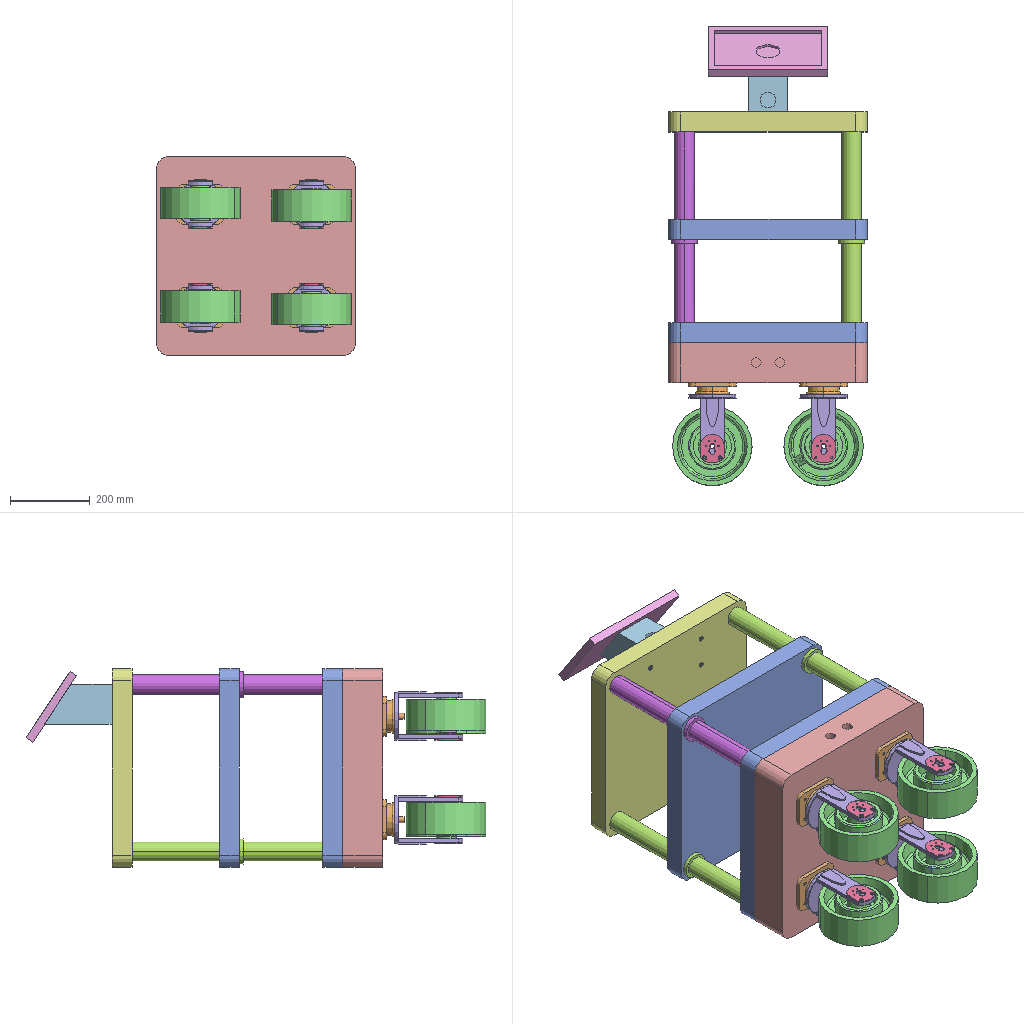Assembly | SolidWorks | 13 different items | 35 placed | box 500 x 1156 x 500 mm
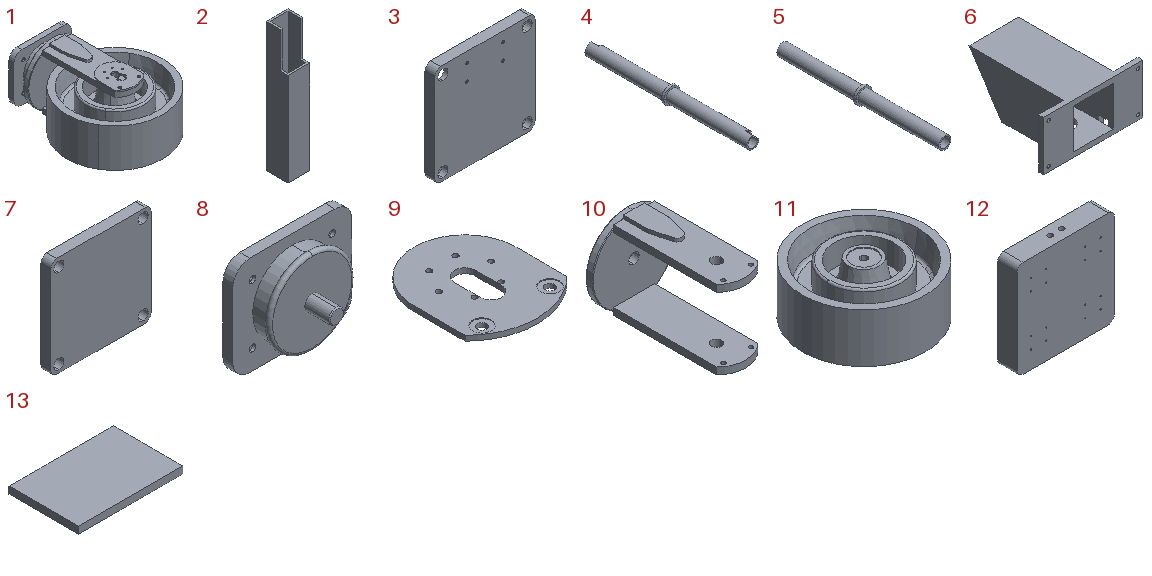Parts list (item | name | quantity | parent item | size | volume | features):
1 | (subassembly) | x4 | - | 200 x 260 x 124 mm | 1930087 mm3 | features CompositeCurve 10, AEMSimFeature 1, MirrorCompFeat 1, ReferencePattern 1
2 | - | x1 | - | 30 x 30 x 180 mm | 43875 mm3 | features ICE 2, Extrusion 1
3 | - | x1 | - | 500 x 50 x 500 mm | 7022317 mm3 | features ICE 3, Extrusion 1, HoleWzd 1
4 | - | x1 | - | 66 x 660 x 66 mm | 470501 mm3 | features ICE 3, Revolution 1
5 | - | x3 | - | 66 x 660 x 66 mm | 481103 mm3 | features ICE 1, Revolution 1
6 | - | x1 | - | 200 x 200 x 100 mm | 682330 mm3 | features ICE 4, Extrusion 1, HoleWzd 1
7 | - | x2 | - | 500 x 50 x 500 mm | 6892126 mm3 | features ICE 2, Extrusion 1
8 | - | x4 | in 1 | 120 x 55 x 100 mm | 210377 mm3 | features ICE 3, Chamfer 1, Extrusion 1, HoleWzd 1, Revolution 1
9 | - | x8 | in 1 | 60 x 72.426 x 3 mm | 9913 mm3 | features Extrusion 1, HoleWzd 1, ICE 1
10 | - | x4 | in 1 | 120 x 172.426 x 124 mm | 314917 mm3 | features ICE 3, MirrorPattern 2, Extrusion 1, Fillet 1, HoleWzd 1
11 | - | x4 | in 1 | 200 x 200 x 87 mm | 1384967 mm3 | features ICE 3, Fillet 2, Extrusion 1, Revolution 1
12 | - | x1 | - | 500 x 100 x 500 mm | 10401596 mm3 | features ICE 4, 3DProfileFeature 1, Extrusion 1, HoleWzd 1, MirrorPattern 1
13 | - | x1 | - | 300 x 200 x 20 mm | 751035 mm3 | features ICE 2, Extrusion 1
Mates (type | each side: item.copy, entity, surface, feature):
In the top assembly
Coincident | 12.1 face plane Cut-Extrude2 | 5.1 face plane Revolve1
Concentric | 12.1 face cylinder Cut-Extrude2 | 5.1 face cylinder Revolve1
Coincident | 12.1 face plane Cut-Extrude1 | assembly face
Concentric | 12.1 face cylinder Cut-Extrude2 | assembly face
Coincident | 12.1 face plane Cut-Extrude2 | 5.2 edge
Concentric | 12.1 face cylinder Cut-Extrude2 | 5.2 face cylinder Revolve1
Coincident | 12.1 face plane Cut-Extrude2 | 5.3 face plane Revolve1
Concentric | 12.1 face cylinder Cut-Extrude2 | 5.3 face cylinder Revolve1
Coincident | 12.1 face plane Boss-Extrude1 | 7.1 face plane Boss-Extrude1
Concentric | 7.1 face cylinder Cut-Extrude2 | assembly face
Concentric | 7.1 face cylinder Cut-Extrude2 | 5.1 face cylinder Revolve1
Concentric | 7.2 face cylinder Cut-Extrude2 | assembly face
Concentric | 7.2 face cylinder Cut-Extrude2 | 5.2 face cylinder Revolve1
Coincident | 5.1 face plane Revolve1 | 7.2 face plane Boss-Extrude1
Coincident | 12.1 face plane Boss-Extrude1 | 8.1 face plane Boss-Extrude1
Concentric | 12.1 face | 8.1 face cylinder CBORE for M6 Hexagon socket head cap screws1
Concentric | 12.1 face | 8.1 edge
Coincident | 13.1 face plane Boss-Extrude1 | 6.1 face plane Cut-Extrude1
Concentric | 5.1 face cylinder Revolve1 | 3.1 face cylinder Cut-Extrude2
Coincident | 2.1 face plane Cut-Extrude3 | 6.1 face plane Boss-Extrude1
Coincident | 2.1 edge | 6.1 edge
Coincident | 6.1 face plane Boss-Extrude1 | 3.1 face plane Cut-Extrude1
Concentric | 6.1 edge | 3.1 face cylinder CBORE for M6 Hexagon head bolts-Full thread-grade C1
Coincident | 2.1 face plane Boss-Extrude1 | 3.1 face plane Cut-Extrude1
Coincident | assembly face | 3.1 face plane Boss-Extrude1
Concentric | 7.2 face cylinder Cut-Extrude2 | 4.1 face cylinder Revolve1
Coincident | 7.2 face plane Boss-Extrude1 | 4.1 face plane Revolve1
In subassembly 1
Concentric | 8.2 edge | 10.1 edge
Coincident | 8.2 face plane Boss-Extrude2 | 10.1 face plane Boss-Extrude1
Concentric | 8.2 edge | 1.1 edge
Coincident | 1.1 face | 10.1 face plane Boss-Extrude1
Parallel | 8.2 face plane Boss-Extrude1 | 10.1 plane
Coincident | 10.1 face plane Mirror2 | 11.1 face plane Revolve1
Coincident | 10.1 face plane Mirror2 | 9.1 face plane Boss-Extrude1
Concentric | 10.1 face cylinder CBORE for M5 Hexagon head bolts-Full thread-grade C1 | 9.1 face cylinder CBORE for M5 Hexagon head bolts-Full thread-grade C1